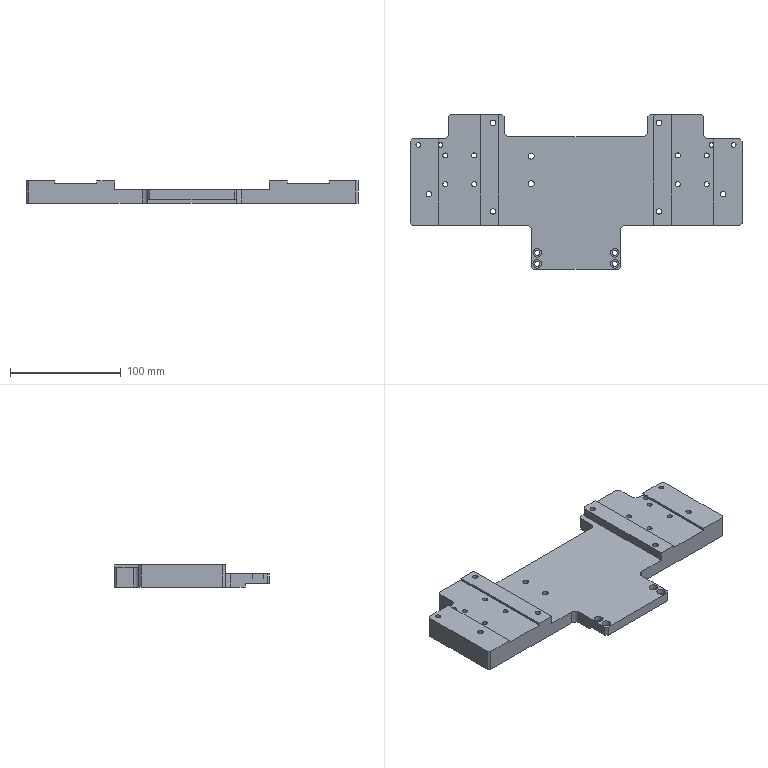Part | SolidWorks | features HoleWzd 7, Chamfer 4, Cut 4, Fillet 3, ICE 2, Extrusion 1 | 1 solid | 157 faces | box 300 x 140 x 20 mm | volume 435356 mm3 | cylinder 90 | plane 59 | cone 8 | commonest cylinder face diameters 4.5 x24 8 x16 5 x12 10 x10 2.5 x8 4.2 x8